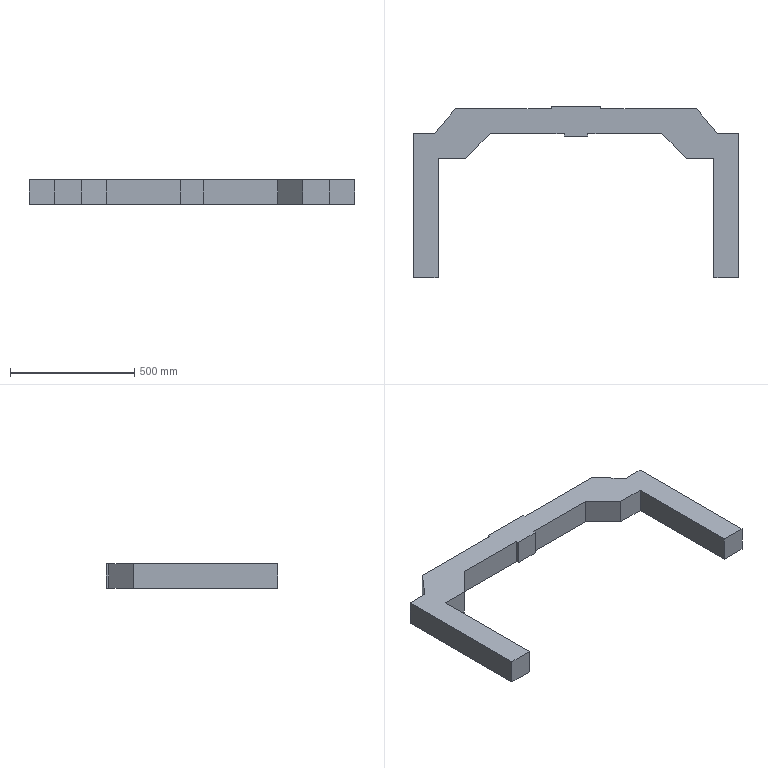Part | SolidWorks | features BaseBody 1 | 1 solid | 32 faces | box 1310 x 690 x 100 mm | volume 25394673 mm3 | plane 28 | cylinder 4 | commonest cylinder face diameters 40 x4
STEP:
#1=CARTESIAN_POINT('',(2389.927,1716.635,30.));
#2=VERTEX_POINT('',#1);
#3=CARTESIAN_POINT('',(2389.927,1716.635,70.));
#4=VERTEX_POINT('',#3);
#5=CARTESIAN_POINT('',(2389.927,1716.635,50.));
#6=DIRECTION('',(0.,1.,0.));
#7=DIRECTION('',(0.,0.,1.));
#8=AXIS2_PLACEMENT_3D('',#5,#6,#7);
#9=CIRCLE('',#8,20.);
#10=EDGE_CURVE('',#2,#4,#9,.T.);
#11=ORIENTED_EDGE('',*,*,#10,.F.);
#12=CARTESIAN_POINT('',(2389.927,1816.635,30.));
#13=VERTEX_POINT('',#12);
#14=CARTESIAN_POINT('',(2389.927,1816.635,30.));
#15=DIRECTION('',(0.,1.,0.));
#16=VECTOR('',#15,1000.);
#17=LINE('',#14,#16);
#18=EDGE_CURVE('',#2,#13,#17,.T.);
#19=ORIENTED_EDGE('',*,*,#18,.T.);
#20=CARTESIAN_POINT('',(2389.927,1816.635,70.));
#21=VERTEX_POINT('',#20);
#22=CARTESIAN_POINT('',(2389.927,1816.635,50.));
#23=DIRECTION('',(0.,1.,0.));
#24=DIRECTION('',(0.,0.,1.));
#25=AXIS2_PLACEMENT_3D('',#22,#23,#24);
#26=CIRCLE('',#25,20.);
#27=EDGE_CURVE('',#13,#21,#26,.T.);
#28=ORIENTED_EDGE('',*,*,#27,.T.);
#29=CARTESIAN_POINT('',(2389.927,1816.635,70.));
#30=DIRECTION('',(0.,1.,0.));
#31=VECTOR('',#30,1000.);
#32=LINE('',#29,#31);
#33=EDGE_CURVE('',#4,#21,#32,.T.);
#34=ORIENTED_EDGE('',*,*,#33,.F.);
#35=EDGE_LOOP('',(#11,#19,#28,#34));
#36=FACE_OUTER_BOUND('',#35,.T.);
#37=CARTESIAN_POINT('',(2389.927,1816.635,50.));
#38=DIRECTION('',(0.,1.,0.));
#39=DIRECTION('',(0.,0.,1.));
#40=AXIS2_PLACEMENT_3D('',#37,#38,#39);
#41=CYLINDRICAL_SURFACE('',#40,20.);
#42=ADVANCED_FACE('',(#36),#41,.F.);
#43=CARTESIAN_POINT('',(3614.927,1716.635,30.));
#44=VERTEX_POINT('',#43);
#45=CARTESIAN_POINT('',(3614.927,1716.635,70.));
#46=VERTEX_POINT('',#45);
#47=CARTESIAN_POINT('',(3614.927,1716.635,50.));
#48=DIRECTION('',(0.,1.,0.));
#49=DIRECTION('',(0.,0.,1.));
#50=AXIS2_PLACEMENT_3D('',#47,#48,#49);
#51=CIRCLE('',#50,20.);
#52=EDGE_CURVE('',#44,#46,#51,.T.);
#53=ORIENTED_EDGE('',*,*,#52,.F.);
#54=CARTESIAN_POINT('',(3614.927,1816.635,30.));
#55=VERTEX_POINT('',#54);
#56=CARTESIAN_POINT('',(3614.927,1816.635,30.));
#57=DIRECTION('',(0.,1.,0.));
#58=VECTOR('',#57,1000.);
#59=LINE('',#56,#58);
#60=EDGE_CURVE('',#44,#55,#59,.T.);
#61=ORIENTED_EDGE('',*,*,#60,.T.);
#62=CARTESIAN_POINT('',(3614.927,1816.635,70.));
#63=VERTEX_POINT('',#62);
#64=CARTESIAN_POINT('',(3614.927,1816.635,50.));
#65=DIRECTION('',(0.,1.,0.));
#66=DIRECTION('',(0.,0.,1.));
#67=AXIS2_PLACEMENT_3D('',#64,#65,#66);
#68=CIRCLE('',#67,20.);
#69=EDGE_CURVE('',#55,#63,#68,.T.);
#70=ORIENTED_EDGE('',*,*,#69,.T.);
#71=CARTESIAN_POINT('',(3614.927,1816.635,70.));
#72=DIRECTION('',(0.,1.,0.));
#73=VECTOR('',#72,1000.);
#74=LINE('',#71,#73);
#75=EDGE_CURVE('',#46,#63,#74,.T.);
#76=ORIENTED_EDGE('',*,*,#75,.F.);
#77=EDGE_LOOP('',(#53,#61,#70,#76));
#78=FACE_OUTER_BOUND('',#77,.T.);
#79=CARTESIAN_POINT('',(3614.927,1816.635,50.));
#80=DIRECTION('',(0.,1.,0.));
#81=DIRECTION('',(0.,0.,1.));
#82=AXIS2_PLACEMENT_3D('',#79,#80,#81);
#83=CYLINDRICAL_SURFACE('',#82,20.);
#84=ADVANCED_FACE('',(#78),#83,.F.);
#85=CARTESIAN_POINT('',(3557.427,1236.635,100.));
#86=VERTEX_POINT('',#85);
#87=CARTESIAN_POINT('',(3557.427,1236.635,0.));
#88=VERTEX_POINT('',#87);
#89=CARTESIAN_POINT('',(3557.427,1236.635,100.));
#90=DIRECTION('',(0.,0.,-1.));
#91=VECTOR('',#90,1000.);
#92=LINE('',#89,#91);
#93=EDGE_CURVE('',#86,#88,#92,.T.);
#94=ORIENTED_EDGE('',*,*,#93,.T.);
#95=CARTESIAN_POINT('',(3657.427,1236.635,0.));
#96=VERTEX_POINT('',#95);
#97=CARTESIAN_POINT('',(2347.427,1236.635,0.));
#98=DIRECTION('',(1.,0.,0.));
#99=VECTOR('',#98,1000.);
#100=LINE('',#97,#99);
#101=EDGE_CURVE('',#88,#96,#100,.T.);
#102=ORIENTED_EDGE('',*,*,#101,.T.);
#103=CARTESIAN_POINT('',(3657.427,1236.635,100.));
#104=VERTEX_POINT('',#103);
#105=CARTESIAN_POINT('',(3657.427,1236.635,0.));
#106=DIRECTION('',(0.,0.,1.));
#107=VECTOR('',#106,1000.);
#108=LINE('',#105,#107);
#109=EDGE_CURVE('',#96,#104,#108,.T.);
#110=ORIENTED_EDGE('',*,*,#109,.T.);
#111=CARTESIAN_POINT('',(2347.427,1236.635,100.));
#112=DIRECTION('',(1.,0.,0.));
#113=VECTOR('',#112,1000.);
#114=LINE('',#111,#113);
#115=EDGE_CURVE('',#86,#104,#114,.T.);
#116=ORIENTED_EDGE('',*,*,#115,.F.);
#117=EDGE_LOOP('',(#94,#102,#110,#116));
#118=FACE_OUTER_BOUND('',#117,.T.);
#119=CARTESIAN_POINT('',(2347.427,1236.635,0.));
#120=DIRECTION('',(0.,-1.,0.));
#121=DIRECTION('',(0.,0.,-1.));
#122=AXIS2_PLACEMENT_3D('',#119,#120,#121);
#123=PLANE('',#122);
#124=ADVANCED_FACE('',(#118),#123,.T.);
#125=CARTESIAN_POINT('',(2447.427,1236.635,100.));
#126=VERTEX_POINT('',#125);
#127=CARTESIAN_POINT('',(2447.427,1236.635,0.));
#128=VERTEX_POINT('',#127);
#129=CARTESIAN_POINT('',(2447.427,1236.635,100.));
#130=DIRECTION('',(0.,0.,-1.));
#131=VECTOR('',#130,1000.);
#132=LINE('',#129,#131);
#133=EDGE_CURVE('',#126,#128,#132,.T.);
#134=ORIENTED_EDGE('',*,*,#133,.F.);
#135=CARTESIAN_POINT('',(2347.427,1236.635,100.));
#136=VERTEX_POINT('',#135);
#137=CARTESIAN_POINT('',(2347.427,1236.635,100.));
#138=DIRECTION('',(1.,0.,0.));
#139=VECTOR('',#138,1000.);
#140=LINE('',#137,#139);
#141=EDGE_CURVE('',#136,#126,#140,.T.);
#142=ORIENTED_EDGE('',*,*,#141,.F.);
#143=CARTESIAN_POINT('',(2347.427,1236.635,0.));
#144=VERTEX_POINT('',#143);
#145=CARTESIAN_POINT('',(2347.427,1236.635,0.));
#146=DIRECTION('',(0.,0.,1.));
#147=VECTOR('',#146,1000.);
#148=LINE('',#145,#147);
#149=EDGE_CURVE('',#144,#136,#148,.T.);
#150=ORIENTED_EDGE('',*,*,#149,.F.);
#151=CARTESIAN_POINT('',(2347.427,1236.635,0.));
#152=DIRECTION('',(1.,0.,0.));
#153=VECTOR('',#152,1000.);
#154=LINE('',#151,#153);
#155=EDGE_CURVE('',#144,#128,#154,.T.);
#156=ORIENTED_EDGE('',*,*,#155,.T.);
#157=EDGE_LOOP('',(#134,#142,#150,#156));
#158=FACE_OUTER_BOUND('',#157,.T.);
#159=CARTESIAN_POINT('',(2347.427,1236.635,0.));
#160=DIRECTION('',(0.,-1.,0.));
#161=DIRECTION('',(0.,0.,-1.));
#162=AXIS2_PLACEMENT_3D('',#159,#160,#161);
#163=PLANE('',#162);
#164=ADVANCED_FACE('',(#158),#163,.T.);
#165=CARTESIAN_POINT('',(2347.427,1816.635,100.));
#166=VERTEX_POINT('',#165);
#167=CARTESIAN_POINT('',(2347.427,1816.635,0.));
#168=VERTEX_POINT('',#167);
#169=CARTESIAN_POINT('',(2347.427,1816.635,100.));
#170=DIRECTION('',(0.,0.,-1.));
#171=VECTOR('',#170,1000.);
#172=LINE('',#169,#171);
#173=EDGE_CURVE('',#166,#168,#172,.T.);
#174=ORIENTED_EDGE('',*,*,#173,.T.);
#175=CARTESIAN_POINT('',(2347.427,1926.635,0.));
#176=DIRECTION('',(0.,-1.,0.));
#177=VECTOR('',#176,1000.);
#178=LINE('',#175,#177);
#179=EDGE_CURVE('',#168,#144,#178,.T.);
#180=ORIENTED_EDGE('',*,*,#179,.T.);
#181=ORIENTED_EDGE('',*,*,#149,.T.);
#182=CARTESIAN_POINT('',(2347.427,1926.635,100.));
#183=DIRECTION('',(0.,-1.,0.));
#184=VECTOR('',#183,1000.);
#185=LINE('',#182,#184);
#186=EDGE_CURVE('',#166,#136,#185,.T.);
#187=ORIENTED_EDGE('',*,*,#186,.F.);
#188=EDGE_LOOP('',(#174,#180,#181,#187));
#189=FACE_OUTER_BOUND('',#188,.T.);
#190=CARTESIAN_POINT('',(2347.427,1926.635,0.));
#191=DIRECTION('',(-1.,0.,0.));
#192=DIRECTION('',(0.,0.,1.));
#193=AXIS2_PLACEMENT_3D('',#190,#191,#192);
#194=PLANE('',#193);
#195=ADVANCED_FACE('',(#189),#194,.T.);
#196=CARTESIAN_POINT('',(2902.427,1926.635,100.));
#197=VERTEX_POINT('',#196);
#198=CARTESIAN_POINT('',(2902.427,1926.635,0.));
#199=VERTEX_POINT('',#198);
#200=CARTESIAN_POINT('',(2902.427,1926.635,100.));
#201=DIRECTION('',(0.,0.,-1.));
#202=VECTOR('',#201,1000.);
#203=LINE('',#200,#202);
#204=EDGE_CURVE('',#197,#199,#203,.T.);
#205=ORIENTED_EDGE('',*,*,#204,.F.);
#206=CARTESIAN_POINT('',(3102.427,1926.635,100.));
#207=VERTEX_POINT('',#206);
#208=CARTESIAN_POINT('',(3657.427,1926.635,100.));
#209=DIRECTION('',(-1.,0.,0.));
#210=VECTOR('',#209,1000.);
#211=LINE('',#208,#210);
#212=EDGE_CURVE('',#207,#197,#211,.T.);
#213=ORIENTED_EDGE('',*,*,#212,.F.);
#214=CARTESIAN_POINT('',(3102.427,1926.635,0.));
#215=VERTEX_POINT('',#214);
#216=CARTESIAN_POINT('',(3102.427,1926.635,100.));
#217=DIRECTION('',(0.,0.,-1.));
#218=VECTOR('',#217,1000.);
#219=LINE('',#216,#218);
#220=EDGE_CURVE('',#207,#215,#219,.T.);
#221=ORIENTED_EDGE('',*,*,#220,.T.);
#222=CARTESIAN_POINT('',(3657.427,1926.635,0.));
#223=DIRECTION('',(-1.,0.,0.));
#224=VECTOR('',#223,1000.);
#225=LINE('',#222,#224);
#226=EDGE_CURVE('',#215,#199,#225,.T.);
#227=ORIENTED_EDGE('',*,*,#226,.T.);
#228=EDGE_LOOP('',(#205,#213,#221,#227));
#229=FACE_OUTER_BOUND('',#228,.T.);
#230=CARTESIAN_POINT('',(3657.427,1926.635,0.));
#231=DIRECTION('',(0.,1.,0.));
#232=DIRECTION('',(0.,0.,1.));
#233=AXIS2_PLACEMENT_3D('',#230,#231,#232);
#234=PLANE('',#233);
#235=ADVANCED_FACE('',(#229),#234,.T.);
#236=CARTESIAN_POINT('',(3657.427,1816.635,100.));
#237=VERTEX_POINT('',#236);
#238=CARTESIAN_POINT('',(3657.427,1816.635,0.));
#239=VERTEX_POINT('',#238);
#240=CARTESIAN_POINT('',(3657.427,1816.635,100.));
#241=DIRECTION('',(0.,0.,-1.));
#242=VECTOR('',#241,1000.);
#243=LINE('',#240,#242);
#244=EDGE_CURVE('',#237,#239,#243,.T.);
#245=ORIENTED_EDGE('',*,*,#244,.F.);
#246=CARTESIAN_POINT('',(3657.427,1236.635,100.));
#247=DIRECTION('',(0.,1.,0.));
#248=VECTOR('',#247,1000.);
#249=LINE('',#246,#248);
#250=EDGE_CURVE('',#104,#237,#249,.T.);
#251=ORIENTED_EDGE('',*,*,#250,.F.);
#252=ORIENTED_EDGE('',*,*,#109,.F.);
#253=CARTESIAN_POINT('',(3657.427,1236.635,0.));
#254=DIRECTION('',(0.,1.,0.));
#255=VECTOR('',#254,1000.);
#256=LINE('',#253,#255);
#257=EDGE_CURVE('',#96,#239,#256,.T.);
#258=ORIENTED_EDGE('',*,*,#257,.T.);
#259=EDGE_LOOP('',(#245,#251,#252,#258));
#260=FACE_OUTER_BOUND('',#259,.T.);
#261=CARTESIAN_POINT('',(3657.427,1236.635,0.));
#262=DIRECTION('',(1.,0.,0.));
#263=DIRECTION('',(0.,0.,-1.));
#264=AXIS2_PLACEMENT_3D('',#261,#262,#263);
#265=PLANE('',#264);
#266=ADVANCED_FACE('',(#260),#265,.T.);
#267=ORIENTED_EDGE('',*,*,#101,.F.);
#268=CARTESIAN_POINT('',(3557.427,1716.635,0.));
#269=VERTEX_POINT('',#268);
#270=CARTESIAN_POINT('',(3557.427,1716.635,0.));
#271=DIRECTION('',(0.,-1.,0.));
#272=VECTOR('',#271,1000.);
#273=LINE('',#270,#272);
#274=EDGE_CURVE('',#269,#88,#273,.T.);
#275=ORIENTED_EDGE('',*,*,#274,.F.);
#276=CARTESIAN_POINT('',(3447.427,1716.635,0.));
#277=VERTEX_POINT('',#276);
#278=CARTESIAN_POINT('',(3447.427,1716.635,0.));
#279=DIRECTION('',(1.,0.,0.));
#280=VECTOR('',#279,1000.);
#281=LINE('',#278,#280);
#282=EDGE_CURVE('',#277,#269,#281,.T.);
#283=ORIENTED_EDGE('',*,*,#282,.F.);
#284=CARTESIAN_POINT('',(3347.427,1816.635,0.));
#285=VERTEX_POINT('',#284);
#286=CARTESIAN_POINT('',(3447.427,1716.635,0.));
#287=DIRECTION('',(0.7071,-0.7071,0.));
#288=VECTOR('',#287,1000.);
#289=LINE('',#286,#288);
#290=EDGE_CURVE('',#285,#277,#289,.T.);
#291=ORIENTED_EDGE('',*,*,#290,.F.);
#292=CARTESIAN_POINT('',(3050.427,1816.635,0.));
#293=VERTEX_POINT('',#292);
#294=CARTESIAN_POINT('',(3050.427,1816.635,0.));
#295=DIRECTION('',(1.,0.,0.));
#296=VECTOR('',#295,1000.);
#297=LINE('',#294,#296);
#298=EDGE_CURVE('',#293,#285,#297,.T.);
#299=ORIENTED_EDGE('',*,*,#298,.F.);
#300=CARTESIAN_POINT('',(3050.427,1806.635,0.));
#301=VERTEX_POINT('',#300);
#302=CARTESIAN_POINT('',(3050.427,1806.635,0.));
#303=DIRECTION('',(0.,1.,0.));
#304=VECTOR('',#303,1000.);
#305=LINE('',#302,#304);
#306=EDGE_CURVE('',#301,#293,#305,.T.);
#307=ORIENTED_EDGE('',*,*,#306,.F.);
#308=CARTESIAN_POINT('',(2954.427,1806.635,0.));
#309=VERTEX_POINT('',#308);
#310=CARTESIAN_POINT('',(2954.427,1806.635,0.));
#311=DIRECTION('',(1.,0.,0.));
#312=VECTOR('',#311,1000.);
#313=LINE('',#310,#312);
#314=EDGE_CURVE('',#309,#301,#313,.T.);
#315=ORIENTED_EDGE('',*,*,#314,.F.);
#316=CARTESIAN_POINT('',(2954.427,1816.635,0.));
#317=VERTEX_POINT('',#316);
#318=CARTESIAN_POINT('',(2954.427,1816.635,0.));
#319=DIRECTION('',(0.,-1.,0.));
#320=VECTOR('',#319,1000.);
#321=LINE('',#318,#320);
#322=EDGE_CURVE('',#317,#309,#321,.T.);
#323=ORIENTED_EDGE('',*,*,#322,.F.);
#324=CARTESIAN_POINT('',(2657.427,1816.635,0.));
#325=VERTEX_POINT('',#324);
#326=CARTESIAN_POINT('',(2657.427,1816.635,0.));
#327=DIRECTION('',(1.,0.,0.));
#328=VECTOR('',#327,1000.);
#329=LINE('',#326,#328);
#330=EDGE_CURVE('',#325,#317,#329,.T.);
#331=ORIENTED_EDGE('',*,*,#330,.F.);
#332=CARTESIAN_POINT('',(2557.427,1716.635,0.));
#333=VERTEX_POINT('',#332);
#334=CARTESIAN_POINT('',(2657.427,1816.635,0.));
#335=DIRECTION('',(0.7071,0.7071,0.));
#336=VECTOR('',#335,1000.);
#337=LINE('',#334,#336);
#338=EDGE_CURVE('',#333,#325,#337,.T.);
#339=ORIENTED_EDGE('',*,*,#338,.F.);
#340=CARTESIAN_POINT('',(2447.427,1716.635,0.));
#341=VERTEX_POINT('',#340);
#342=CARTESIAN_POINT('',(2447.427,1716.635,0.));
#343=DIRECTION('',(1.,0.,0.));
#344=VECTOR('',#343,1000.);
#345=LINE('',#342,#344);
#346=EDGE_CURVE('',#341,#333,#345,.T.);
#347=ORIENTED_EDGE('',*,*,#346,.F.);
#348=CARTESIAN_POINT('',(2447.427,1236.635,0.));
#349=DIRECTION('',(0.,1.,0.));
#350=VECTOR('',#349,1000.);
#351=LINE('',#348,#350);
#352=EDGE_CURVE('',#128,#341,#351,.T.);
#353=ORIENTED_EDGE('',*,*,#352,.F.);
#354=ORIENTED_EDGE('',*,*,#155,.F.);
#355=ORIENTED_EDGE('',*,*,#179,.F.);
#356=CARTESIAN_POINT('',(2432.427,1816.635,0.));
#357=VERTEX_POINT('',#356);
#358=CARTESIAN_POINT('',(2432.427,1816.635,0.));
#359=DIRECTION('',(-1.,0.,0.));
#360=VECTOR('',#359,1000.);
#361=LINE('',#358,#360);
#362=EDGE_CURVE('',#357,#168,#361,.T.);
#363=ORIENTED_EDGE('',*,*,#362,.F.);
#364=CARTESIAN_POINT('',(2517.427,1916.635,0.));
#365=VERTEX_POINT('',#364);
#366=CARTESIAN_POINT('',(2432.427,1816.635,0.));
#367=DIRECTION('',(-0.6476,-0.7619,0.));
#368=VECTOR('',#367,1000.);
#369=LINE('',#366,#368);
#370=EDGE_CURVE('',#365,#357,#369,.T.);
#371=ORIENTED_EDGE('',*,*,#370,.F.);
#372=CARTESIAN_POINT('',(2902.427,1916.635,0.));
#373=VERTEX_POINT('',#372);
#374=CARTESIAN_POINT('',(2902.427,1916.635,0.));
#375=DIRECTION('',(-1.,0.,0.));
#376=VECTOR('',#375,1000.);
#377=LINE('',#374,#376);
#378=EDGE_CURVE('',#373,#365,#377,.T.);
#379=ORIENTED_EDGE('',*,*,#378,.F.);
#380=CARTESIAN_POINT('',(2902.427,1926.635,0.));
#381=DIRECTION('',(0.,-1.,0.));
#382=VECTOR('',#381,1000.);
#383=LINE('',#380,#382);
#384=EDGE_CURVE('',#199,#373,#383,.T.);
#385=ORIENTED_EDGE('',*,*,#384,.F.);
#386=ORIENTED_EDGE('',*,*,#226,.F.);
#387=CARTESIAN_POINT('',(3102.427,1916.635,0.));
#388=VERTEX_POINT('',#387);
#389=CARTESIAN_POINT('',(3102.427,1916.635,0.));
#390=DIRECTION('',(0.,1.,0.));
#391=VECTOR('',#390,1000.);
#392=LINE('',#389,#391);
#393=EDGE_CURVE('',#388,#215,#392,.T.);
#394=ORIENTED_EDGE('',*,*,#393,.F.);
#395=CARTESIAN_POINT('',(3487.427,1916.635,0.));
#396=VERTEX_POINT('',#395);
#397=CARTESIAN_POINT('',(3487.427,1916.635,0.));
#398=DIRECTION('',(-1.,0.,0.));
#399=VECTOR('',#398,1000.);
#400=LINE('',#397,#399);
#401=EDGE_CURVE('',#396,#388,#400,.T.);
#402=ORIENTED_EDGE('',*,*,#401,.F.);
#403=CARTESIAN_POINT('',(3572.427,1816.635,0.));
#404=VERTEX_POINT('',#403);
#405=CARTESIAN_POINT('',(3487.427,1916.635,0.));
#406=DIRECTION('',(-0.6476,0.7619,0.));
#407=VECTOR('',#406,1000.);
#408=LINE('',#405,#407);
#409=EDGE_CURVE('',#404,#396,#408,.T.);
#410=ORIENTED_EDGE('',*,*,#409,.F.);
#411=CARTESIAN_POINT('',(3657.427,1816.635,0.));
#412=DIRECTION('',(-1.,0.,0.));
#413=VECTOR('',#412,1000.);
#414=LINE('',#411,#413);
#415=EDGE_CURVE('',#239,#404,#414,.T.);
#416=ORIENTED_EDGE('',*,*,#415,.F.);
#417=ORIENTED_EDGE('',*,*,#257,.F.);
#418=EDGE_LOOP('',(#267,#275,#283,#291,#299,#307,#315,#323,#331,#339,#347,#353,#354,#355,#363,#371,#379,#385,#386,#394,#402,#410,#416,#417));
#419=FACE_OUTER_BOUND('',#418,.T.);
#420=CARTESIAN_POINT('',(0.,0.,0.));
#421=DIRECTION('',(0.,0.,1.));
#422=DIRECTION('',(1.,0.,0.));
#423=AXIS2_PLACEMENT_3D('',#420,#421,#422);
#424=PLANE('',#423);
#425=ADVANCED_FACE('',(#419),#424,.F.);
#426=CARTESIAN_POINT('',(3557.427,1716.635,100.));
#427=VERTEX_POINT('',#426);
#428=CARTESIAN_POINT('',(3557.427,1716.635,100.));
#429=DIRECTION('',(0.,-1.,0.));
#430=VECTOR('',#429,1000.);
#431=LINE('',#428,#430);
#432=EDGE_CURVE('',#427,#86,#431,.T.);
#433=ORIENTED_EDGE('',*,*,#432,.T.);
#434=ORIENTED_EDGE('',*,*,#115,.T.);
#435=ORIENTED_EDGE('',*,*,#250,.T.);
#436=CARTESIAN_POINT('',(3572.427,1816.635,100.));
#437=VERTEX_POINT('',#436);
#438=CARTESIAN_POINT('',(3657.427,1816.635,100.));
#439=DIRECTION('',(-1.,0.,0.));
#440=VECTOR('',#439,1000.);
#441=LINE('',#438,#440);
#442=EDGE_CURVE('',#237,#437,#441,.T.);
#443=ORIENTED_EDGE('',*,*,#442,.T.);
#444=CARTESIAN_POINT('',(3487.427,1916.635,100.));
#445=VERTEX_POINT('',#444);
#446=CARTESIAN_POINT('',(3487.427,1916.635,100.));
#447=DIRECTION('',(-0.6476,0.7619,0.));
#448=VECTOR('',#447,1000.);
#449=LINE('',#446,#448);
#450=EDGE_CURVE('',#437,#445,#449,.T.);
#451=ORIENTED_EDGE('',*,*,#450,.T.);
#452=CARTESIAN_POINT('',(3102.427,1916.635,100.));
#453=VERTEX_POINT('',#452);
#454=CARTESIAN_POINT('',(3487.427,1916.635,100.));
#455=DIRECTION('',(-1.,0.,0.));
#456=VECTOR('',#455,1000.);
#457=LINE('',#454,#456);
#458=EDGE_CURVE('',#445,#453,#457,.T.);
#459=ORIENTED_EDGE('',*,*,#458,.T.);
#460=CARTESIAN_POINT('',(3102.427,1916.635,100.));
#461=DIRECTION('',(0.,1.,0.));
#462=VECTOR('',#461,1000.);
#463=LINE('',#460,#462);
#464=EDGE_CURVE('',#453,#207,#463,.T.);
#465=ORIENTED_EDGE('',*,*,#464,.T.);
#466=ORIENTED_EDGE('',*,*,#212,.T.);
#467=CARTESIAN_POINT('',(2902.427,1916.635,100.));
#468=VERTEX_POINT('',#467);
#469=CARTESIAN_POINT('',(2902.427,1926.635,100.));
#470=DIRECTION('',(0.,-1.,0.));
#471=VECTOR('',#470,1000.);
#472=LINE('',#469,#471);
#473=EDGE_CURVE('',#197,#468,#472,.T.);
#474=ORIENTED_EDGE('',*,*,#473,.T.);
#475=CARTESIAN_POINT('',(2517.427,1916.635,100.));
#476=VERTEX_POINT('',#475);
#477=CARTESIAN_POINT('',(2902.427,1916.635,100.));
#478=DIRECTION('',(-1.,0.,0.));
#479=VECTOR('',#478,1000.);
#480=LINE('',#477,#479);
#481=EDGE_CURVE('',#468,#476,#480,.T.);
#482=ORIENTED_EDGE('',*,*,#481,.T.);
#483=CARTESIAN_POINT('',(2432.427,1816.635,100.));
#484=VERTEX_POINT('',#483);
#485=CARTESIAN_POINT('',(2432.427,1816.635,100.));
#486=DIRECTION('',(-0.6476,-0.7619,0.));
#487=VECTOR('',#486,1000.);
#488=LINE('',#485,#487);
#489=EDGE_CURVE('',#476,#484,#488,.T.);
#490=ORIENTED_EDGE('',*,*,#489,.T.);
#491=CARTESIAN_POINT('',(2432.427,1816.635,100.));
#492=DIRECTION('',(-1.,0.,0.));
#493=VECTOR('',#492,1000.);
#494=LINE('',#491,#493);
#495=EDGE_CURVE('',#484,#166,#494,.T.);
#496=ORIENTED_EDGE('',*,*,#495,.T.);
#497=ORIENTED_EDGE('',*,*,#186,.T.);
#498=ORIENTED_EDGE('',*,*,#141,.T.);
#499=CARTESIAN_POINT('',(2447.427,1716.635,100.));
#500=VERTEX_POINT('',#499);
#501=CARTESIAN_POINT('',(2447.427,1236.635,100.));
#502=DIRECTION('',(0.,1.,0.));
#503=VECTOR('',#502,1000.);
#504=LINE('',#501,#503);
#505=EDGE_CURVE('',#126,#500,#504,.T.);
#506=ORIENTED_EDGE('',*,*,#505,.T.);
#507=CARTESIAN_POINT('',(2557.427,1716.635,100.));
#508=VERTEX_POINT('',#507);
#509=CARTESIAN_POINT('',(2447.427,1716.635,100.));
#510=DIRECTION('',(1.,0.,0.));
#511=VECTOR('',#510,1000.);
#512=LINE('',#509,#511);
#513=EDGE_CURVE('',#500,#508,#512,.T.);
#514=ORIENTED_EDGE('',*,*,#513,.T.);
#515=CARTESIAN_POINT('',(2657.427,1816.635,100.));
#516=VERTEX_POINT('',#515);
#517=CARTESIAN_POINT('',(2657.427,1816.635,100.));
#518=DIRECTION('',(0.7071,0.7071,0.));
#519=VECTOR('',#518,1000.);
#520=LINE('',#517,#519);
#521=EDGE_CURVE('',#508,#516,#520,.T.);
#522=ORIENTED_EDGE('',*,*,#521,.T.);
#523=CARTESIAN_POINT('',(2954.427,1816.635,100.));
#524=VERTEX_POINT('',#523);
#525=CARTESIAN_POINT('',(2657.427,1816.635,100.));
#526=DIRECTION('',(1.,0.,0.));
#527=VECTOR('',#526,1000.);
#528=LINE('',#525,#527);
#529=EDGE_CURVE('',#516,#524,#528,.T.);
#530=ORIENTED_EDGE('',*,*,#529,.T.);
#531=CARTESIAN_POINT('',(2954.427,1806.635,100.));
#532=VERTEX_POINT('',#531);
#533=CARTESIAN_POINT('',(2954.427,1816.635,100.));
#534=DIRECTION('',(0.,-1.,0.));
#535=VECTOR('',#534,1000.);
#536=LINE('',#533,#535);
#537=EDGE_CURVE('',#524,#532,#536,.T.);
#538=ORIENTED_EDGE('',*,*,#537,.T.);
#539=CARTESIAN_POINT('',(3050.427,1806.635,100.));
#540=VERTEX_POINT('',#539);
#541=CARTESIAN_POINT('',(2954.427,1806.635,100.));
#542=DIRECTION('',(1.,0.,0.));
#543=VECTOR('',#542,1000.);
#544=LINE('',#541,#543);
#545=EDGE_CURVE('',#532,#540,#544,.T.);
#546=ORIENTED_EDGE('',*,*,#545,.T.);
#547=CARTESIAN_POINT('',(3050.427,1816.635,100.));
#548=VERTEX_POINT('',#547);
#549=CARTESIAN_POINT('',(3050.427,1806.635,100.));
#550=DIRECTION('',(0.,1.,0.));
#551=VECTOR('',#550,1000.);
#552=LINE('',#549,#551);
#553=EDGE_CURVE('',#540,#548,#552,.T.);
#554=ORIENTED_EDGE('',*,*,#553,.T.);
#555=CARTESIAN_POINT('',(3347.427,1816.635,100.));
#556=VERTEX_POINT('',#555);
#557=CARTESIAN_POINT('',(3050.427,1816.635,100.));
#558=DIRECTION('',(1.,0.,0.));
#559=VECTOR('',#558,1000.);
#560=LINE('',#557,#559);
#561=EDGE_CURVE('',#548,#556,#560,.T.);
#562=ORIENTED_EDGE('',*,*,#561,.T.);
#563=CARTESIAN_POINT('',(3447.427,1716.635,100.));
#564=VERTEX_POINT('',#563);
#565=CARTESIAN_POINT('',(3447.427,1716.635,100.));
#566=DIRECTION('',(0.7071,-0.7071,0.));
#567=VECTOR('',#566,1000.);
#568=LINE('',#565,#567);
#569=EDGE_CURVE('',#556,#564,#568,.T.);
#570=ORIENTED_EDGE('',*,*,#569,.T.);
#571=CARTESIAN_POINT('',(3447.427,1716.635,100.));
#572=DIRECTION('',(1.,0.,0.));
#573=VECTOR('',#572,1000.);
#574=LINE('',#571,#573);
#575=EDGE_CURVE('',#564,#427,#574,.T.);
#576=ORIENTED_EDGE('',*,*,#575,.T.);
#577=EDGE_LOOP('',(#433,#434,#435,#443,#451,#459,#465,#466,#474,#482,#490,#496,#497,#498,#506,#514,#522,#530,#538,#546,#554,#562,#570,#576));
#578=FACE_OUTER_BOUND('',#577,.T.);
#579=CARTESIAN_POINT('',(0.,0.,100.));
#580=DIRECTION('',(0.,0.,1.));
#581=DIRECTION('',(1.,0.,0.));
#582=AXIS2_PLACEMENT_3D('',#579,#580,#581);
#583=PLANE('',#582);
#584=ADVANCED_FACE('',(#578),#583,.T.);
#585=ORIENTED_EDGE('',*,*,#409,.T.);
#586=CARTESIAN_POINT('',(3487.427,1916.635,100.));
#587=DIRECTION('',(0.,0.,-1.));
#588=VECTOR('',#587,1000.);
#589=LINE('',#586,#588);
#590=EDGE_CURVE('',#445,#396,#589,.T.);
#591=ORIENTED_EDGE('',*,*,#590,.F.);
#592=ORIENTED_EDGE('',*,*,#450,.F.);
#593=CARTESIAN_POINT('',(3572.427,1816.635,100.));
#594=DIRECTION('',(0.,0.,-1.));
#595=VECTOR('',#594,1000.);
#596=LINE('',#593,#595);
#597=EDGE_CURVE('',#437,#404,#596,.T.);
#598=ORIENTED_EDGE('',*,*,#597,.T.);
#599=EDGE_LOOP('',(#585,#591,#592,#598));
#600=FACE_OUTER_BOUND('',#599,.T.);
#601=CARTESIAN_POINT('',(3487.427,1916.635,100.));
#602=DIRECTION('',(0.7619,0.6476,0.));
#603=DIRECTION('',(-0.6476,0.7619,0.));
#604=AXIS2_PLACEMENT_3D('',#601,#602,#603);
#605=PLANE('',#604);
#606=ADVANCED_FACE('',(#600),#605,.T.);
#607=CARTESIAN_POINT('',(3614.927,1816.635,50.));
#608=DIRECTION('',(0.,1.,0.));
#609=DIRECTION('',(0.,0.,1.));
#610=AXIS2_PLACEMENT_3D('',#607,#608,#609);
#611=CIRCLE('',#610,20.);
#612=EDGE_CURVE('',#63,#55,#611,.T.);
#613=ORIENTED_EDGE('',*,*,#612,.F.);
#614=ORIENTED_EDGE('',*,*,#69,.F.);
#615=EDGE_LOOP('',(#613,#614));
#616=FACE_BOUND('',#615,.T.);
#617=ORIENTED_EDGE('',*,*,#415,.T.);
#618=ORIENTED_EDGE('',*,*,#597,.F.);
#619=ORIENTED_EDGE('',*,*,#442,.F.);
#620=ORIENTED_EDGE('',*,*,#244,.T.);
#621=EDGE_LOOP('',(#617,#618,#619,#620));
#622=FACE_OUTER_BOUND('',#621,.T.);
#623=CARTESIAN_POINT('',(3657.427,1816.635,100.));
#624=DIRECTION('',(0.,-1.,0.));
#625=DIRECTION('',(0.,0.,-1.));
#626=AXIS2_PLACEMENT_3D('',#623,#624,#625);
#627=PLANE('',#626);
#628=ADVANCED_FACE('',(#616,#622),#627,.F.);
#629=ORIENTED_EDGE('',*,*,#393,.T.);
#630=ORIENTED_EDGE('',*,*,#220,.F.);
#631=ORIENTED_EDGE('',*,*,#464,.F.);
#632=CARTESIAN_POINT('',(3102.427,1916.635,100.));
#633=DIRECTION('',(0.,0.,-1.));
#634=VECTOR('',#633,1000.);
#635=LINE('',#632,#634);
#636=EDGE_CURVE('',#453,#388,#635,.T.);
#637=ORIENTED_EDGE('',*,*,#636,.T.);
#638=EDGE_LOOP('',(#629,#630,#631,#637));
#639=FACE_OUTER_BOUND('',#638,.T.);
#640=CARTESIAN_POINT('',(3102.427,1916.635,100.));
#641=DIRECTION('',(-1.,0.,0.));
#642=DIRECTION('',(0.,-1.,0.));
#643=AXIS2_PLACEMENT_3D('',#640,#641,#642);
#644=PLANE('',#643);
#645=ADVANCED_FACE('',(#639),#644,.F.);
#646=ORIENTED_EDGE('',*,*,#401,.T.);
#647=ORIENTED_EDGE('',*,*,#636,.F.);
#648=ORIENTED_EDGE('',*,*,#458,.F.);
#649=ORIENTED_EDGE('',*,*,#590,.T.);
#650=EDGE_LOOP('',(#646,#647,#648,#649));
#651=FACE_OUTER_BOUND('',#650,.T.);
#652=CARTESIAN_POINT('',(3487.427,1916.635,100.));
#653=DIRECTION('',(0.,-1.,0.));
#654=DIRECTION('',(1.,0.,0.));
#655=AXIS2_PLACEMENT_3D('',#652,#653,#654);
#656=PLANE('',#655);
#657=ADVANCED_FACE('',(#651),#656,.F.);
#658=ORIENTED_EDGE('',*,*,#378,.T.);
#659=CARTESIAN_POINT('',(2517.427,1916.635,100.));
#660=DIRECTION('',(0.,0.,-1.));
#661=VECTOR('',#660,1000.);
#662=LINE('',#659,#661);
#663=EDGE_CURVE('',#476,#365,#662,.T.);
#664=ORIENTED_EDGE('',*,*,#663,.F.);
#665=ORIENTED_EDGE('',*,*,#481,.F.);
#666=CARTESIAN_POINT('',(2902.427,1916.635,100.));
#667=DIRECTION('',(0.,0.,-1.));
#668=VECTOR('',#667,1000.);
#669=LINE('',#666,#668);
#670=EDGE_CURVE('',#468,#373,#669,.T.);
#671=ORIENTED_EDGE('',*,*,#670,.T.);
#672=EDGE_LOOP('',(#658,#664,#665,#671));
#673=FACE_OUTER_BOUND('',#672,.T.);
#674=CARTESIAN_POINT('',(2902.427,1916.635,100.));
#675=DIRECTION('',(0.,-1.,0.));
#676=DIRECTION('',(1.,0.,0.));
#677=AXIS2_PLACEMENT_3D('',#674,#675,#676);
#678=PLANE('',#677);
#679=ADVANCED_FACE('',(#673),#678,.F.);
#680=ORIENTED_EDGE('',*,*,#384,.T.);
#681=ORIENTED_EDGE('',*,*,#670,.F.);
#682=ORIENTED_EDGE('',*,*,#473,.F.);
#683=ORIENTED_EDGE('',*,*,#204,.T.);
#684=EDGE_LOOP('',(#680,#681,#682,#683));
#685=FACE_OUTER_BOUND('',#684,.T.);
#686=CARTESIAN_POINT('',(2902.427,1926.635,100.));
#687=DIRECTION('',(1.,0.,0.));
#688=DIRECTION('',(0.,0.,-1.));
#689=AXIS2_PLACEMENT_3D('',#686,#687,#688);
#690=PLANE('',#689);
#691=ADVANCED_FACE('',(#685),#690,.F.);
#692=CARTESIAN_POINT('',(2389.927,1816.635,50.));
#693=DIRECTION('',(0.,1.,0.));
#694=DIRECTION('',(0.,0.,1.));
#695=AXIS2_PLACEMENT_3D('',#692,#693,#694);
#696=CIRCLE('',#695,20.);
#697=EDGE_CURVE('',#21,#13,#696,.T.);
#698=ORIENTED_EDGE('',*,*,#697,.F.);
#699=ORIENTED_EDGE('',*,*,#27,.F.);
#700=EDGE_LOOP('',(#698,#699));
#701=FACE_BOUND('',#700,.T.);
#702=ORIENTED_EDGE('',*,*,#362,.T.);
#703=ORIENTED_EDGE('',*,*,#173,.F.);
#704=ORIENTED_EDGE('',*,*,#495,.F.);
#705=CARTESIAN_POINT('',(2432.427,1816.635,100.));
#706=DIRECTION('',(0.,0.,-1.));
#707=VECTOR('',#706,1000.);
#708=LINE('',#705,#707);
#709=EDGE_CURVE('',#484,#357,#708,.T.);
#710=ORIENTED_EDGE('',*,*,#709,.T.);
#711=EDGE_LOOP('',(#702,#703,#704,#710));
#712=FACE_OUTER_BOUND('',#711,.T.);
#713=CARTESIAN_POINT('',(2432.427,1816.635,100.));
#714=DIRECTION('',(0.,-1.,0.));
#715=DIRECTION('',(0.,0.,-1.));
#716=AXIS2_PLACEMENT_3D('',#713,#714,#715);
#717=PLANE('',#716);
#718=ADVANCED_FACE('',(#701,#712),#717,.F.);
#719=ORIENTED_EDGE('',*,*,#370,.T.);
#720=ORIENTED_EDGE('',*,*,#709,.F.);
#721=ORIENTED_EDGE('',*,*,#489,.F.);
#722=ORIENTED_EDGE('',*,*,#663,.T.);
#723=EDGE_LOOP('',(#719,#720,#721,#722));
#724=FACE_OUTER_BOUND('',#723,.T.);
#725=CARTESIAN_POINT('',(2432.427,1816.635,100.));
#726=DIRECTION('',(-0.7619,0.6476,0.));
#727=DIRECTION('',(-0.6476,-0.7619,0.));
#728=AXIS2_PLACEMENT_3D('',#725,#726,#727);
#729=PLANE('',#728);
#730=ADVANCED_FACE('',(#724),#729,.T.);
#731=ORIENTED_EDGE('',*,*,#274,.T.);
#732=ORIENTED_EDGE('',*,*,#93,.F.);
#733=ORIENTED_EDGE('',*,*,#432,.F.);
#734=CARTESIAN_POINT('',(3557.427,1716.635,100.));
#735=DIRECTION('',(0.,0.,-1.));
#736=VECTOR('',#735,1000.);
#737=LINE('',#734,#736);
#738=EDGE_CURVE('',#427,#269,#737,.T.);
#739=ORIENTED_EDGE('',*,*,#738,.T.);
#740=EDGE_LOOP('',(#731,#732,#733,#739));
#741=FACE_OUTER_BOUND('',#740,.T.);
#742=CARTESIAN_POINT('',(3557.427,1716.635,100.));
#743=DIRECTION('',(1.,0.,0.));
#744=DIRECTION('',(0.,0.,-1.));
#745=AXIS2_PLACEMENT_3D('',#742,#743,#744);
#746=PLANE('',#745);
#747=ADVANCED_FACE('',(#741),#746,.F.);
#748=ORIENTED_EDGE('',*,*,#282,.T.);
#749=ORIENTED_EDGE('',*,*,#738,.F.);
#750=ORIENTED_EDGE('',*,*,#575,.F.);
#751=CARTESIAN_POINT('',(3447.427,1716.635,100.));
#752=DIRECTION('',(0.,0.,-1.));
#753=VECTOR('',#752,1000.);
#754=LINE('',#751,#753);
#755=EDGE_CURVE('',#564,#277,#754,.T.);
#756=ORIENTED_EDGE('',*,*,#755,.T.);
#757=EDGE_LOOP('',(#748,#749,#750,#756));
#758=FACE_OUTER_BOUND('',#757,.T.);
#759=CARTESIAN_POINT('',(3447.427,1716.635,100.));
#760=DIRECTION('',(0.,1.,0.));
#761=DIRECTION('',(0.,0.,1.));
#762=AXIS2_PLACEMENT_3D('',#759,#760,#761);
#763=PLANE('',#762);
#764=ADVANCED_FACE('',(#758),#763,.F.);
#765=ORIENTED_EDGE('',*,*,#290,.T.);
#766=ORIENTED_EDGE('',*,*,#755,.F.);
#767=ORIENTED_EDGE('',*,*,#569,.F.);
#768=CARTESIAN_POINT('',(3347.427,1816.635,100.));
#769=DIRECTION('',(0.,0.,-1.));
#770=VECTOR('',#769,1000.);
#771=LINE('',#768,#770);
#772=EDGE_CURVE('',#556,#285,#771,.T.);
#773=ORIENTED_EDGE('',*,*,#772,.T.);
#774=EDGE_LOOP('',(#765,#766,#767,#773));
#775=FACE_OUTER_BOUND('',#774,.T.);
#776=CARTESIAN_POINT('',(3447.427,1716.635,100.));
#777=DIRECTION('',(-0.7071,-0.7071,0.));
#778=DIRECTION('',(0.7071,-0.7071,0.));
#779=AXIS2_PLACEMENT_3D('',#776,#777,#778);
#780=PLANE('',#779);
#781=ADVANCED_FACE('',(#775),#780,.T.);
#782=ORIENTED_EDGE('',*,*,#298,.T.);
#783=ORIENTED_EDGE('',*,*,#772,.F.);
#784=ORIENTED_EDGE('',*,*,#561,.F.);
#785=CARTESIAN_POINT('',(3050.427,1816.635,100.));
#786=DIRECTION('',(0.,0.,-1.));
#787=VECTOR('',#786,1000.);
#788=LINE('',#785,#787);
#789=EDGE_CURVE('',#548,#293,#788,.T.);
#790=ORIENTED_EDGE('',*,*,#789,.T.);
#791=EDGE_LOOP('',(#782,#783,#784,#790));
#792=FACE_OUTER_BOUND('',#791,.T.);
#793=CARTESIAN_POINT('',(3050.427,1816.635,100.));
#794=DIRECTION('',(0.,1.,0.));
#795=DIRECTION('',(0.,0.,1.));
#796=AXIS2_PLACEMENT_3D('',#793,#794,#795);
#797=PLANE('',#796);
#798=ADVANCED_FACE('',(#792),#797,.F.);
#799=ORIENTED_EDGE('',*,*,#306,.T.);
#800=ORIENTED_EDGE('',*,*,#789,.F.);
#801=ORIENTED_EDGE('',*,*,#553,.F.);
#802=CARTESIAN_POINT('',(3050.427,1806.635,100.));
#803=DIRECTION('',(0.,0.,-1.));
#804=VECTOR('',#803,1000.);
#805=LINE('',#802,#804);
#806=EDGE_CURVE('',#540,#301,#805,.T.);
#807=ORIENTED_EDGE('',*,*,#806,.T.);
#808=EDGE_LOOP('',(#799,#800,#801,#807));
#809=FACE_OUTER_BOUND('',#808,.T.);
#810=CARTESIAN_POINT('',(3050.427,1806.635,100.));
#811=DIRECTION('',(-1.,0.,0.));
#812=DIRECTION('',(0.,0.,1.));
#813=AXIS2_PLACEMENT_3D('',#810,#811,#812);
#814=PLANE('',#813);
#815=ADVANCED_FACE('',(#809),#814,.F.);
#816=ORIENTED_EDGE('',*,*,#314,.T.);
#817=ORIENTED_EDGE('',*,*,#806,.F.);
#818=ORIENTED_EDGE('',*,*,#545,.F.);
#819=CARTESIAN_POINT('',(2954.427,1806.635,100.));
#820=DIRECTION('',(0.,0.,-1.));
#821=VECTOR('',#820,1000.);
#822=LINE('',#819,#821);
#823=EDGE_CURVE('',#532,#309,#822,.T.);
#824=ORIENTED_EDGE('',*,*,#823,.T.);
#825=EDGE_LOOP('',(#816,#817,#818,#824));
#826=FACE_OUTER_BOUND('',#825,.T.);
#827=CARTESIAN_POINT('',(2954.427,1806.635,100.));
#828=DIRECTION('',(0.,1.,0.));
#829=DIRECTION('',(0.,0.,1.));
#830=AXIS2_PLACEMENT_3D('',#827,#828,#829);
#831=PLANE('',#830);
#832=ADVANCED_FACE('',(#826),#831,.F.);
#833=ORIENTED_EDGE('',*,*,#322,.T.);
#834=ORIENTED_EDGE('',*,*,#823,.F.);
#835=ORIENTED_EDGE('',*,*,#537,.F.);
#836=CARTESIAN_POINT('',(2954.427,1816.635,100.));
#837=DIRECTION('',(0.,0.,-1.));
#838=VECTOR('',#837,1000.);
#839=LINE('',#836,#838);
#840=EDGE_CURVE('',#524,#317,#839,.T.);
#841=ORIENTED_EDGE('',*,*,#840,.T.);
#842=EDGE_LOOP('',(#833,#834,#835,#841));
#843=FACE_OUTER_BOUND('',#842,.T.);
#844=CARTESIAN_POINT('',(2954.427,1816.635,100.));
#845=DIRECTION('',(1.,0.,0.));
#846=DIRECTION('',(0.,0.,-1.));
#847=AXIS2_PLACEMENT_3D('',#844,#845,#846);
#848=PLANE('',#847);
#849=ADVANCED_FACE('',(#843),#848,.F.);
#850=ORIENTED_EDGE('',*,*,#330,.T.);
#851=ORIENTED_EDGE('',*,*,#840,.F.);
#852=ORIENTED_EDGE('',*,*,#529,.F.);
#853=CARTESIAN_POINT('',(2657.427,1816.635,100.));
#854=DIRECTION('',(0.,0.,-1.));
#855=VECTOR('',#854,1000.);
#856=LINE('',#853,#855);
#857=EDGE_CURVE('',#516,#325,#856,.T.);
#858=ORIENTED_EDGE('',*,*,#857,.T.);
#859=EDGE_LOOP('',(#850,#851,#852,#858));
#860=FACE_OUTER_BOUND('',#859,.T.);
#861=CARTESIAN_POINT('',(2657.427,1816.635,100.));
#862=DIRECTION('',(0.,1.,0.));
#863=DIRECTION('',(0.,0.,1.));
#864=AXIS2_PLACEMENT_3D('',#861,#862,#863);
#865=PLANE('',#864);
#866=ADVANCED_FACE('',(#860),#865,.F.);
#867=ORIENTED_EDGE('',*,*,#338,.T.);
#868=ORIENTED_EDGE('',*,*,#857,.F.);
#869=ORIENTED_EDGE('',*,*,#521,.F.);
#870=CARTESIAN_POINT('',(2557.427,1716.635,100.));
#871=DIRECTION('',(0.,0.,-1.));
#872=VECTOR('',#871,1000.);
#873=LINE('',#870,#872);
#874=EDGE_CURVE('',#508,#333,#873,.T.);
#875=ORIENTED_EDGE('',*,*,#874,.T.);
#876=EDGE_LOOP('',(#867,#868,#869,#875));
#877=FACE_OUTER_BOUND('',#876,.T.);
#878=CARTESIAN_POINT('',(2657.427,1816.635,100.));
#879=DIRECTION('',(0.7071,-0.7071,0.));
#880=DIRECTION('',(0.7071,0.7071,0.));
#881=AXIS2_PLACEMENT_3D('',#878,#879,#880);
#882=PLANE('',#881);
#883=ADVANCED_FACE('',(#877),#882,.T.);
#884=ORIENTED_EDGE('',*,*,#346,.T.);
#885=ORIENTED_EDGE('',*,*,#874,.F.);
#886=ORIENTED_EDGE('',*,*,#513,.F.);
#887=CARTESIAN_POINT('',(2447.427,1716.635,100.));
#888=DIRECTION('',(0.,0.,-1.));
#889=VECTOR('',#888,1000.);
#890=LINE('',#887,#889);
#891=EDGE_CURVE('',#500,#341,#890,.T.);
#892=ORIENTED_EDGE('',*,*,#891,.T.);
#893=EDGE_LOOP('',(#884,#885,#886,#892));
#894=FACE_OUTER_BOUND('',#893,.T.);
#895=CARTESIAN_POINT('',(2447.427,1716.635,100.));
#896=DIRECTION('',(0.,1.,0.));
#897=DIRECTION('',(0.,0.,1.));
#898=AXIS2_PLACEMENT_3D('',#895,#896,#897);
#899=PLANE('',#898);
#900=ADVANCED_FACE('',(#894),#899,.F.);
#901=ORIENTED_EDGE('',*,*,#352,.T.);
#902=ORIENTED_EDGE('',*,*,#891,.F.);
#903=ORIENTED_EDGE('',*,*,#505,.F.);
#904=ORIENTED_EDGE('',*,*,#133,.T.);
#905=EDGE_LOOP('',(#901,#902,#903,#904));
#906=FACE_OUTER_BOUND('',#905,.T.);
#907=CARTESIAN_POINT('',(2447.427,1236.635,100.));
#908=DIRECTION('',(-1.,0.,0.));
#909=DIRECTION('',(0.,0.,1.));
#910=AXIS2_PLACEMENT_3D('',#907,#908,#909);
#911=PLANE('',#910);
#912=ADVANCED_FACE('',(#906),#911,.F.);
#913=CARTESIAN_POINT('',(3614.927,1716.635,50.));
#914=DIRECTION('',(0.,1.,0.));
#915=DIRECTION('',(0.,0.,1.));
#916=AXIS2_PLACEMENT_3D('',#913,#914,#915);
#917=CIRCLE('',#916,20.);
#918=EDGE_CURVE('',#46,#44,#917,.T.);
#919=ORIENTED_EDGE('',*,*,#918,.T.);
#920=ORIENTED_EDGE('',*,*,#52,.T.);
#921=EDGE_LOOP('',(#919,#920));
#922=FACE_OUTER_BOUND('',#921,.T.);
#923=CARTESIAN_POINT('',(3614.927,1716.635,50.));
#924=DIRECTION('',(0.,-1.,0.));
#925=DIRECTION('',(0.,0.,-1.));
#926=AXIS2_PLACEMENT_3D('',#923,#924,#925);
#927=PLANE('',#926);
#928=ADVANCED_FACE('',(#922),#927,.F.);
#929=ORIENTED_EDGE('',*,*,#60,.F.);
#930=ORIENTED_EDGE('',*,*,#918,.F.);
#931=ORIENTED_EDGE('',*,*,#75,.T.);
#932=ORIENTED_EDGE('',*,*,#612,.T.);
#933=EDGE_LOOP('',(#929,#930,#931,#932));
#934=FACE_OUTER_BOUND('',#933,.T.);
#935=CARTESIAN_POINT('',(3614.927,1816.635,50.));
#936=DIRECTION('',(0.,1.,0.));
#937=DIRECTION('',(0.,0.,1.));
#938=AXIS2_PLACEMENT_3D('',#935,#936,#937);
#939=CYLINDRICAL_SURFACE('',#938,20.);
#940=ADVANCED_FACE('',(#934),#939,.F.);
#941=CARTESIAN_POINT('',(2389.927,1716.635,50.));
#942=DIRECTION('',(0.,1.,0.));
#943=DIRECTION('',(0.,0.,1.));
#944=AXIS2_PLACEMENT_3D('',#941,#942,#943);
#945=CIRCLE('',#944,20.);
#946=EDGE_CURVE('',#4,#2,#945,.T.);
#947=ORIENTED_EDGE('',*,*,#946,.T.);
#948=ORIENTED_EDGE('',*,*,#10,.T.);
#949=EDGE_LOOP('',(#947,#948));
#950=FACE_OUTER_BOUND('',#949,.T.);
#951=CARTESIAN_POINT('',(2389.927,1716.635,50.));
#952=DIRECTION('',(0.,-1.,0.));
#953=DIRECTION('',(0.,0.,-1.));
#954=AXIS2_PLACEMENT_3D('',#951,#952,#953);
#955=PLANE('',#954);
#956=ADVANCED_FACE('',(#950),#955,.F.);
#957=ORIENTED_EDGE('',*,*,#18,.F.);
#958=ORIENTED_EDGE('',*,*,#946,.F.);
#959=ORIENTED_EDGE('',*,*,#33,.T.);
#960=ORIENTED_EDGE('',*,*,#697,.T.);
#961=EDGE_LOOP('',(#957,#958,#959,#960));
#962=FACE_OUTER_BOUND('',#961,.T.);
#963=CARTESIAN_POINT('',(2389.927,1816.635,50.));
#964=DIRECTION('',(0.,1.,0.));
#965=DIRECTION('',(0.,0.,1.));
#966=AXIS2_PLACEMENT_3D('',#963,#964,#965);
#967=CYLINDRICAL_SURFACE('',#966,20.);
#968=ADVANCED_FACE('',(#962),#967,.F.);
#969=CLOSED_SHELL('',(#42,#84,#124,#164,#195,#235,#266,#425,#584,#606,#628,#645,#657,#679,#691,#718,#730,#747,#764,#781,#798,#815,#832,#849,#866,#883,#900,#912,#928,#940,#956,#968));
#970=MANIFOLD_SOLID_BREP('',#969);
#971=CARTESIAN_POINT('',(0.,0.,0.));
#972=DIRECTION('',(0.,0.,1.));
#973=DIRECTION('',(1.,0.,0.));
#974=AXIS2_PLACEMENT_3D('',#971,#972,#973);
#975=(LENGTH_UNIT()NAMED_UNIT(*)SI_UNIT(.MILLI.,.METRE.));
#976=UNCERTAINTY_MEASURE_WITH_UNIT(LENGTH_MEASURE(0.00001),#975,'','');
#977=(NAMED_UNIT(*)PLANE_ANGLE_UNIT()SI_UNIT($,.RADIAN.));
#978=(NAMED_UNIT(*)SI_UNIT($,.STERADIAN.)SOLID_ANGLE_UNIT());
#979=(GEOMETRIC_REPRESENTATION_CONTEXT(3)GLOBAL_UNCERTAINTY_ASSIGNED_CONTEXT((#976))GLOBAL_UNIT_ASSIGNED_CONTEXT((#975,#977,#978))REPRESENTATION_CONTEXT('',''));
#980=ADVANCED_BREP_SHAPE_REPRESENTATION('',(#970,#974),#979);